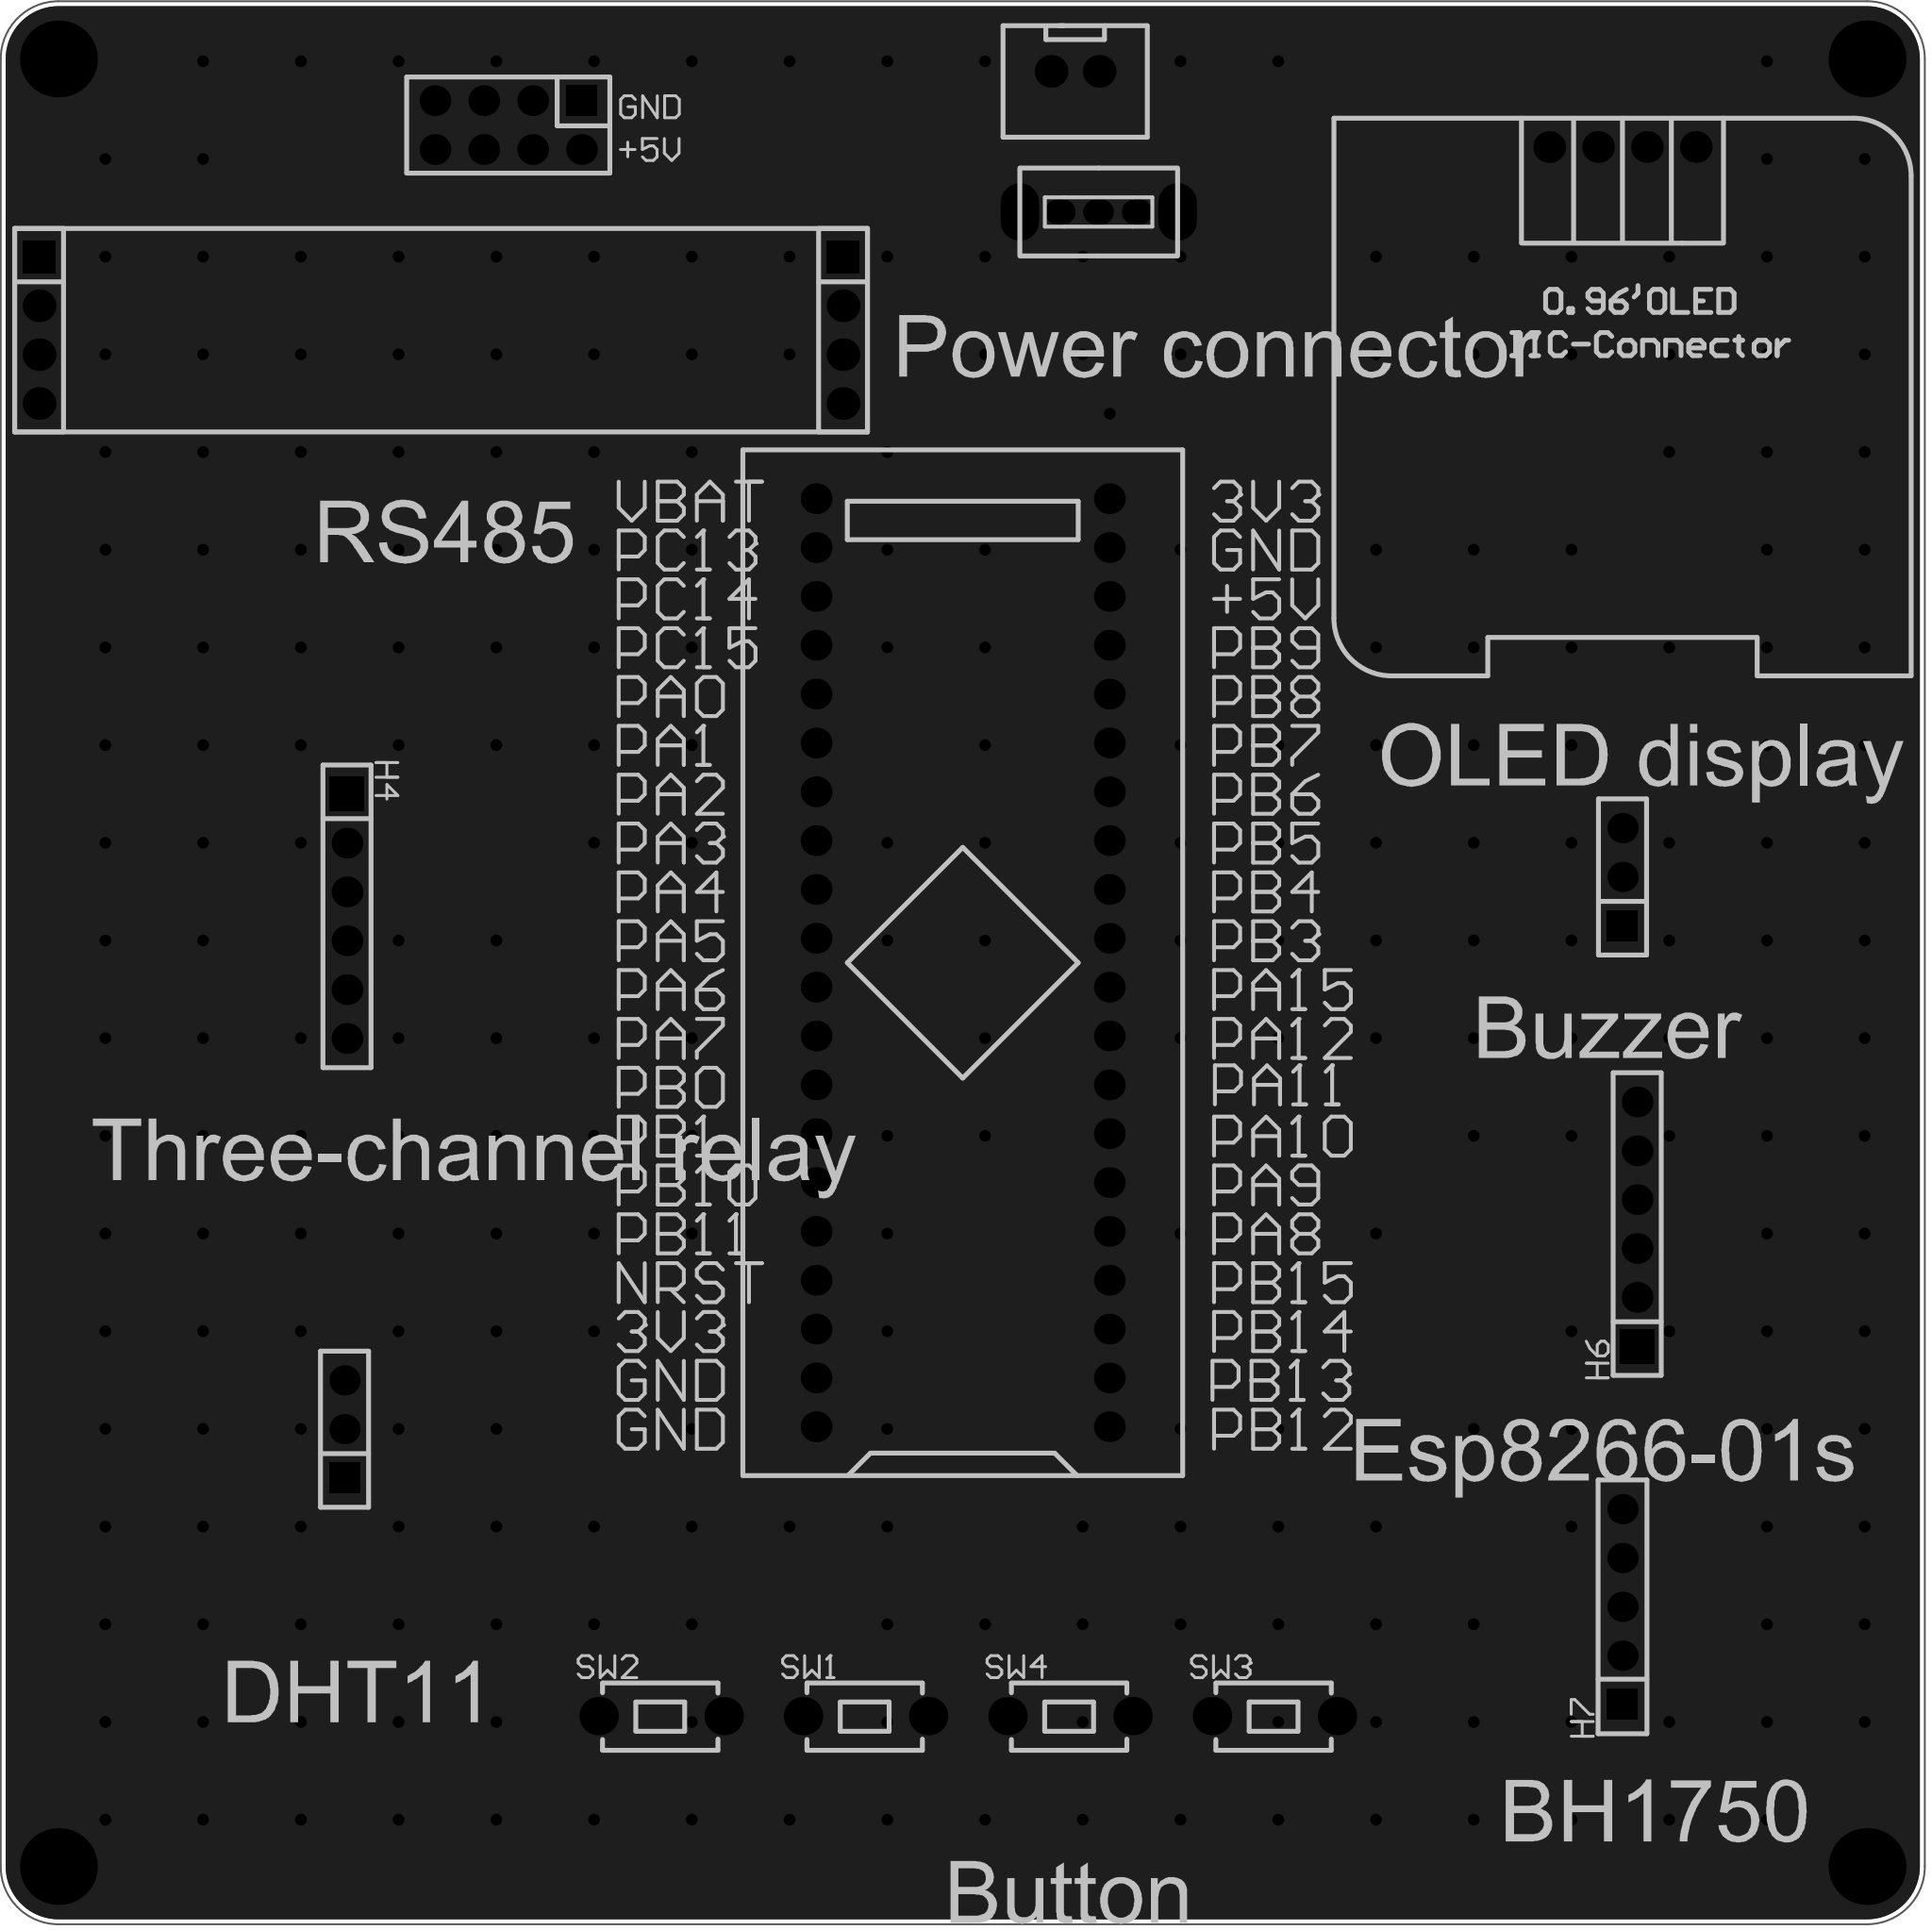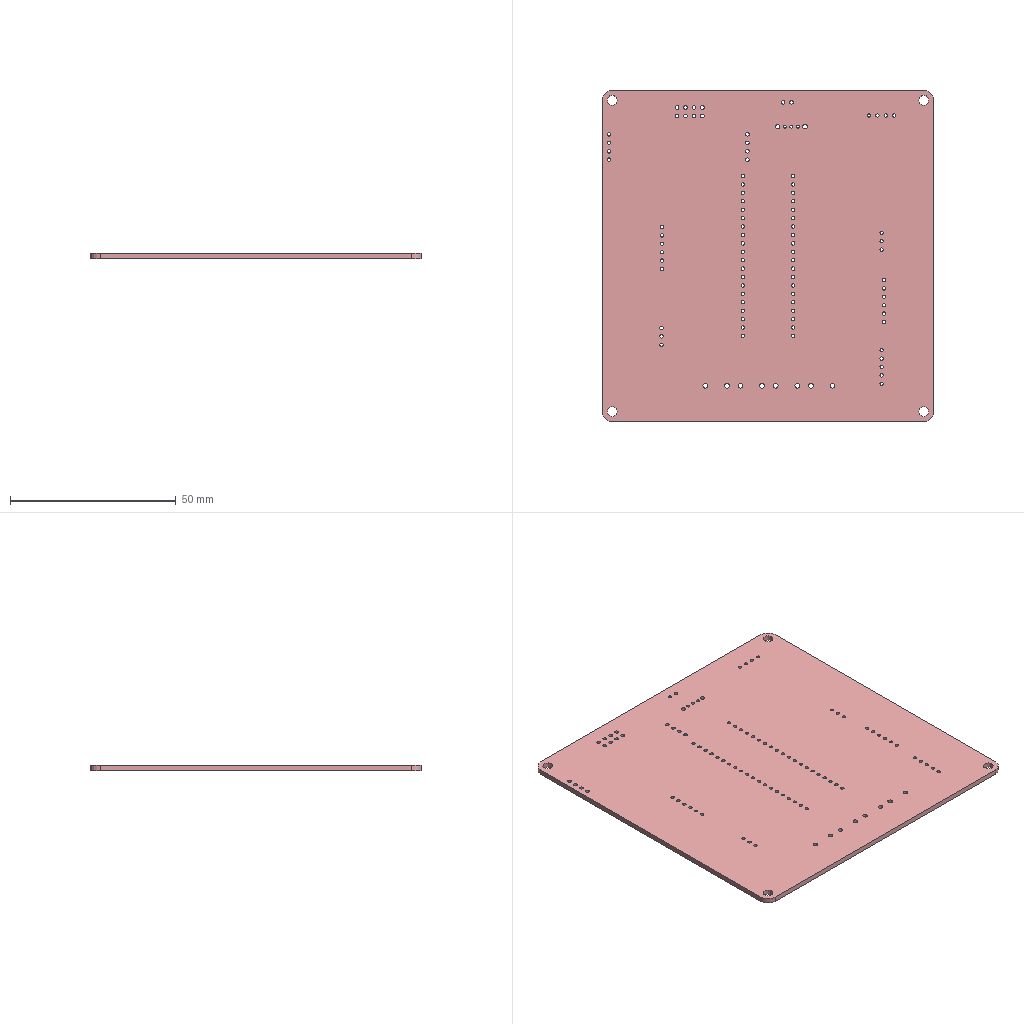Circuit board layout | Altium Designer | box 100 x 100 x 1.6 mm
Layer stack:
# Altium Designer layer stack of  (unit mm; dielectric type: 0 none, 1 core, 2 prepreg, 3 surface material)
index,name,kind,layer,copper_thickness_mm,dielectric_type,dielectric_thickness_mm,dielectric_material,dielectric_constant
0,Top Paste Mask Layer,other,,,,,,
1,Top Silkscreen Layer,other,,,,,,
2,Top Solder Mask Layer,dielectric,,,3,0.01,,3.3
3,Top Layer,copper,Top Layer,0.035,,,,
4,Dielectric1,dielectric,,,3,1.51,FR4,4.5
5,Bottom Layer,copper,Bottom Layer,0.035,,,,
6,Bottom Solder Mask Layer,dielectric,,,3,0.01,,3.3
7,Bottom Silkscreen Layer,other,,,,,,
8,Bottom Paste Mask Layer,other,,,,,,
# drill layer pairs: low layer,high layer
drill_pair,Top Layer,Bottom Layer
Part placement:
Designator,Comment,Layer,Footprint,Center-X(mm),Center-Y(mm),Rotation
U1,STM32F103C8T6-Card,TopLayer,CONN-TH_L53.3-W22.9_STM32F103C8T6-CARD,141.351,130.937,90
OLED1,,TopLayer,0.96OLED_4P,175.641,173.355,0
CN4,XH2.54*2P_Straight,TopLayer,CONN-TH_2P-P2.50-XH2.54-2P,147.193,177.292,0
SW5,,TopLayer,拨动开关,148.417,169.978,0
H1,,TopLayer,HDR-TH_3P-P2.54-V-F,175.641,135.399,90
H3,,TopLayer,HDR-TH_3P-P2.54-V-F,109.22,106.68,90
H5,,TopLayer,HDR-TH_4P-P2.54-V-F,135.128,163.83,270
H7,,TopLayer,HDR-TH_5P-P2.54-V-F,175.641,97.442,90
SW1,,TopLayer,Key_TH_3.5x6x4.3,136.303,91.76,0
SW2,,TopLayer,Key_TH_3.5x6x4.3,125.677,91.76,0
SW3,,TopLayer,Key_TH_3.5x6x4.3,157.554,91.76,0
SW4,,TopLayer,Key_TH_3.5x6x4.3,146.929,91.76,0
H2,,TopLayer,HDR-TH_4P-P2.54-V-F,93.345,163.83,270
H4,,TopLayer,HDR-TH_6P-P2.54-V-F,109.347,133.35,270
H6,,TopLayer,HDR-TH_6P-P2.54-V-F,176.403,117.348,90
H8,,TopLayer,HDR-TH_8P-P2.54-V-F-R2-C4-S2.54-1,117.729,174.498,180
Pad and via stacks:
# Altium Designer via and pad stacks of  (unit mm). Each distinct definition once, with the count of objects using it.
# via: kind,start_layer,end_layer,hole_mm,diameter_mm,mode(0 simple;1 top-mid-bottom;2 full stack),diameter_per_layer,count,example_net
# pad: kind,layer,hole_mm,hole_type(0 round;1 square;2 slot),plating,top_size,top_shape(1 round;2 rect;3 octagon;9 rounded rect),mid_size,bottom_size,mode,footprint,size_per_layer,count,example
pad,Multi-Layer,3,0,plated,4x4,1,4x4,4x4,0,,,4,1
pad,Multi-Layer,1,0,plated,1.6x1.6,1,1.6x1.6,1.6x1.6,0,CONN-TH_L53.3-W22.9_STM32F103C8T6-CARD,,40,U1.1
pad,Multi-Layer,1,0,plated,1.65x1.65,1,1.65x1.65,1.65x1.65,0,0.96OLED_4P,,4,OLED1.4
pad,Multi-Layer,1.05,0,plated,1.7x1.7,1,1.7x1.7,1.7x1.7,0,CONN-TH_2P-P2.50-XH2.54-2P,,2,CN4.2
pad,Multi-Layer,0.8992,0,plated,1.6x1.3,1,1.6x1.3,1.6x1.3,0,\u00B2\u00A6\u00B6\u00AF\u00BF\u00AA\u00B9\u00D8,,3,SW5.1
pad,Multi-Layer,1.3,0,plated,3x1.999,1,3x1.999,3x1.999,0,\u00B2\u00A6\u00B6\u00AF\u00BF\u00AA\u00B9\u00D8,,2,SW5.4
pad,Multi-Layer,1.02,0,plated,1.575x1.575,1,1.575x1.575,1.575x1.575,0,HDR-TH_3P-P2.54-V-F,,4,H1.3
pad,Multi-Layer,1.02,0,plated,1.575x1.575,2,1.575x1.575,1.575x1.575,0,HDR-TH_3P-P2.54-V-F,,2,H1.1
pad,Multi-Layer,1.1,0,plated,1.7x1.7,2,1.7x1.7,1.7x1.7,0,HDR-TH_4P-P2.54-V-F,,2,H5.1
pad,Multi-Layer,1.1,0,plated,1.7x1.7,1,1.7x1.7,1.7x1.7,0,HDR-TH_4P-P2.54-V-F,,6,H5.2
pad,Multi-Layer,1.02,0,plated,1.575x1.575,1,1.575x1.575,1.575x1.575,0,HDR-TH_5P-P2.54-V-F,,4,H7.5
pad,Multi-Layer,1.02,0,plated,1.575x1.575,2,1.575x1.575,1.575x1.575,0,HDR-TH_5P-P2.54-V-F,,1,H7.1
pad,Multi-Layer,1.399,0,plated,1.999x1.999,1,1.999x1.999,1.999x1.999,0,Key_TH_3.5x6x4.3,,8,SW1.A
pad,Multi-Layer,1.02,0,plated,1.6x1.6,1,1.6x1.6,1.6x1.6,0,HDR-TH_6P-P2.54-V-F,,10,H4.6
pad,Multi-Layer,1.02,0,plated,1.8x1.8,2,1.8x1.8,1.8x1.8,0,HDR-TH_6P-P2.54-V-F,,2,H4.1
pad,Multi-Layer,1.1,0,plated,1.6x1.6,2,1.6x1.6,1.6x1.6,0,HDR-TH_8P-P2.54-V-F-R2-C4-S2.54-1,,1,H8.1
pad,Multi-Layer,1.1,0,plated,1.6x1.6,1,1.6x1.6,1.6x1.6,0,HDR-TH_8P-P2.54-V-F-R2-C4-S2.54-1,,7,H8.2
via,Top Layer,Bottom Layer,0.3048,0.61,0,,269,VCC
Copper pours:
name,layer,net,type(0 solid;1 hatched;2 none)
Bottom Layer-GND,Bottom Layer,GND,0
Top Layer-GND,Top Layer,GND,0
Design rules, without the lines most boards share:
# Altium Designer design rules of  (exported by Altium Designer, unit mm)
# columns: name | kind | enabled | priority | scope1 | scope2 | descriptor | typed fields (field=value)
Copper_copperRegion_copperThickness1oz | 0 | disabled | 4 | All | All | Clearance Constraint (Gap=5.984mil) (Disabled)(All),(All) | gap=0.152
Copper_copperRegion_copperThickness1oz_1 | 63 | disabled | 4 | All | All | Board Clearance Constraint (Gap=0mil) (Disabled)(All) |
Copper_copperRegion_Copper_copperRegion | 0 | disabled | 5 | All | All | Clearance Constraint (Gap=5.984mil) (Disabled)(All),(All) | gap=0.152
Copper_copperRegion_Copper_copperRegion_1 | 63 | disabled | 5 | All | All | Board Clearance Constraint (Gap=0mil) (Disabled)(All) |
copperThickness1oz | 0 | enabled | 6 | All | All | Clearance Constraint (Gap=5.984mil) (All),(All) | gap=0.152
copperThickness1oz_1 | 63 | enabled | 6 | All | All | Board Clearance Constraint (Gap=0mil) (All) |
copperRegion_copperThickness1oz | 20 | disabled | 1 | All | All | Polygon Connect Rule(Relief Connect )(Conductor Width=10mil) (Relief Angle=90 Angle) (Entries=4) (Air Gap Width=10mil) (Disabled)(All),(All) | connect_style(0=relief,1=direct,2=none)=0 relief_conductor_width=0.254 relief_entries=4
copperRegion_Copper_copperRegion | 20 | disabled | 2 | All | All | Polygon Connect Rule(Relief Connect )(Conductor Width=10mil) (Relief Angle=90 Angle) (Entries=4) (Air Gap Width=10mil) (Disabled)(All),(All) | connect_style(0=relief,1=direct,2=none)=0 relief_conductor_width=0.254 relief_entries=4
copperRegion | 20 | enabled | 3 | All | All | Polygon Connect Rule(Relief Connect )(Conductor Width=10mil) (Relief Angle=90 Angle) (Entries=4) (Air Gap Width=10mil) (All),(All) | connect_style(0=relief,1=direct,2=none)=0 relief_conductor_width=0.254 relief_entries=4